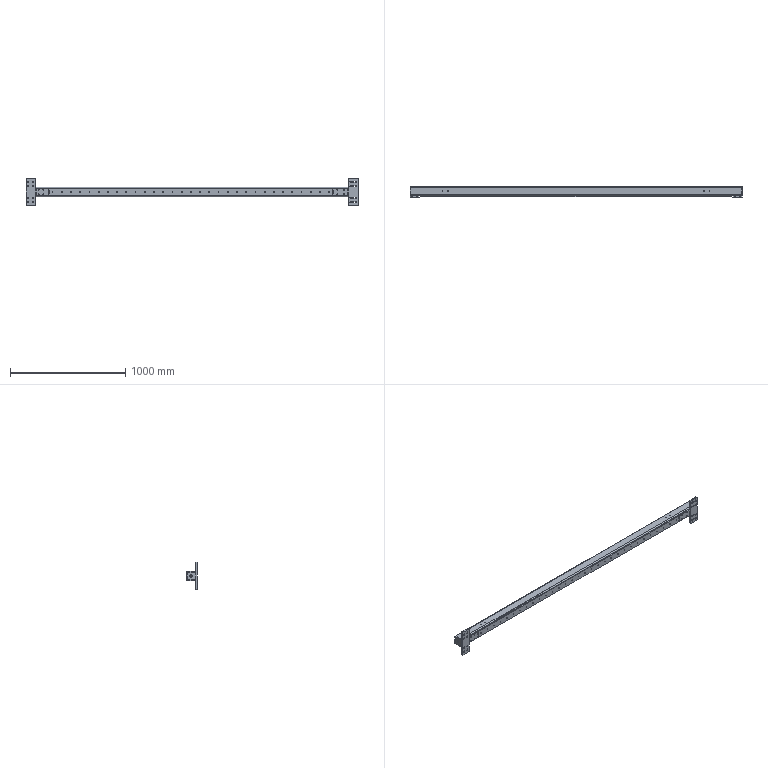Part | SolidWorks | features BaseBody 6 | 6 solids | 418 faces | box 2880 x 95 x 240 mm | volume 7048256 mm3 | cylinder 314 | plane 88 | cone 16 | commonest cylinder face diameters 6.8 x172 5 x40 4.2 x34 9 x24 15 x16 20 x16